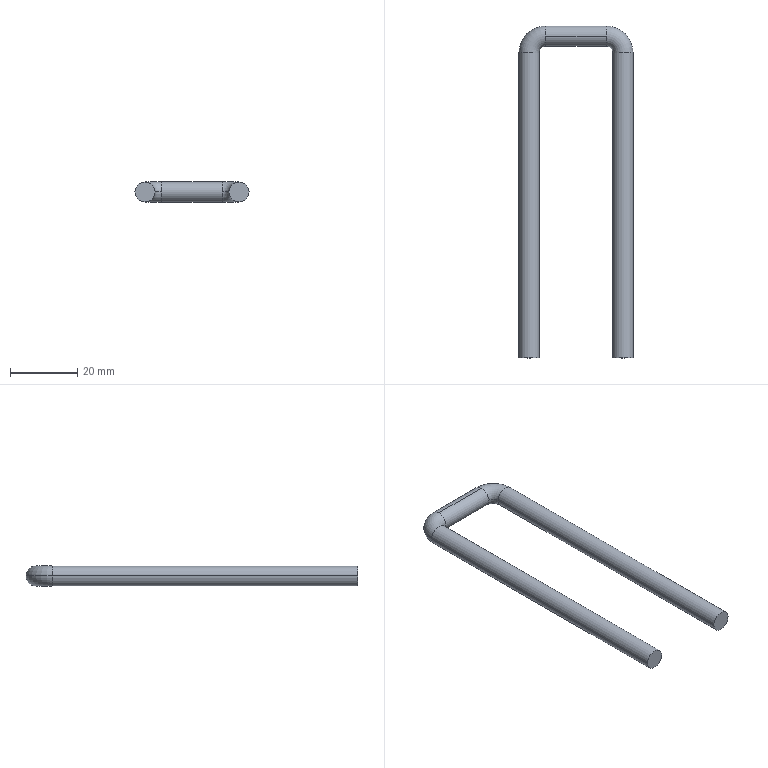Part | SolidWorks | features Sweep 1 | 1 solid | 12 faces | box 34 x 99 x 6 mm | volume 6099 mm3 | cylinder 6 | torus 4 | plane 2 | commonest cylinder face diameters 6 x6
STEP:
#1=CARTESIAN_POINT('',(-11.,91.,0.));
#2=VERTEX_POINT('',#1);
#3=CARTESIAN_POINT('',(-17.,91.,0.));
#4=VERTEX_POINT('',#3);
#5=CARTESIAN_POINT('',(-14.,91.,0.));
#6=DIRECTION('',(0.,1.,0.));
#7=DIRECTION('',(0.,0.,1.));
#8=AXIS2_PLACEMENT_3D('',#5,#6,#7);
#9=CIRCLE('',#8,3.);
#10=EDGE_CURVE('',#2,#4,#9,.T.);
#11=ORIENTED_EDGE('',*,*,#10,.T.);
#12=CARTESIAN_POINT('',(-9.,99.,0.));
#13=VERTEX_POINT('',#12);
#14=CARTESIAN_POINT('',(-9.,91.,0.));
#15=DIRECTION('',(0.,0.,-1.));
#16=DIRECTION('',(0.,1.,0.));
#17=AXIS2_PLACEMENT_3D('',#14,#15,#16);
#18=CIRCLE('',#17,8.);
#19=EDGE_CURVE('',#4,#13,#18,.T.);
#20=ORIENTED_EDGE('',*,*,#19,.T.);
#21=CARTESIAN_POINT('',(-9.,96.,-3.));
#22=VERTEX_POINT('',#21);
#23=CARTESIAN_POINT('',(-9.,96.,0.));
#24=DIRECTION('',(1.,0.,0.));
#25=DIRECTION('',(0.,0.,1.));
#26=AXIS2_PLACEMENT_3D('',#23,#24,#25);
#27=CIRCLE('',#26,3.);
#28=EDGE_CURVE('',#22,#13,#27,.T.);
#29=ORIENTED_EDGE('',*,*,#28,.F.);
#30=CARTESIAN_POINT('',(-9.,93.,0.));
#31=VERTEX_POINT('',#30);
#32=CARTESIAN_POINT('',(-9.,96.,0.));
#33=DIRECTION('',(1.,0.,0.));
#34=DIRECTION('',(0.,0.,1.));
#35=AXIS2_PLACEMENT_3D('',#32,#33,#34);
#36=CIRCLE('',#35,3.);
#37=EDGE_CURVE('',#31,#22,#36,.T.);
#38=ORIENTED_EDGE('',*,*,#37,.F.);
#39=CARTESIAN_POINT('',(-9.,91.,0.));
#40=DIRECTION('',(0.,0.,-1.));
#41=DIRECTION('',(0.,1.,0.));
#42=AXIS2_PLACEMENT_3D('',#39,#40,#41);
#43=CIRCLE('',#42,2.);
#44=EDGE_CURVE('',#2,#31,#43,.T.);
#45=ORIENTED_EDGE('',*,*,#44,.F.);
#46=EDGE_LOOP('',(#11,#20,#29,#38,#45));
#47=FACE_OUTER_BOUND('',#46,.T.);
#48=CARTESIAN_POINT('',(-9.,91.,0.));
#49=DIRECTION('',(0.,0.,-1.));
#50=DIRECTION('',(-1.,0.,0.));
#51=AXIS2_PLACEMENT_3D('',#48,#49,#50);
#52=TOROIDAL_SURFACE('',#51,5.,3.);
#53=ADVANCED_FACE('',(#47),#52,.T.);
#54=CARTESIAN_POINT('',(9.,96.,-3.));
#55=VERTEX_POINT('',#54);
#56=CARTESIAN_POINT('',(9.,99.,0.));
#57=VERTEX_POINT('',#56);
#58=CARTESIAN_POINT('',(9.,96.,0.));
#59=DIRECTION('',(1.,0.,0.));
#60=DIRECTION('',(0.,0.,1.));
#61=AXIS2_PLACEMENT_3D('',#58,#59,#60);
#62=CIRCLE('',#61,3.);
#63=EDGE_CURVE('',#55,#57,#62,.T.);
#64=ORIENTED_EDGE('',*,*,#63,.T.);
#65=CARTESIAN_POINT('',(17.,91.,0.));
#66=VERTEX_POINT('',#65);
#67=CARTESIAN_POINT('',(9.,91.,0.));
#68=DIRECTION('',(0.,0.,-1.));
#69=DIRECTION('',(0.,1.,0.));
#70=AXIS2_PLACEMENT_3D('',#67,#68,#69);
#71=CIRCLE('',#70,8.);
#72=EDGE_CURVE('',#57,#66,#71,.T.);
#73=ORIENTED_EDGE('',*,*,#72,.T.);
#74=CARTESIAN_POINT('',(11.,91.,0.));
#75=VERTEX_POINT('',#74);
#76=CARTESIAN_POINT('',(14.,91.,0.));
#77=DIRECTION('',(0.,-1.,0.));
#78=DIRECTION('',(0.,0.,1.));
#79=AXIS2_PLACEMENT_3D('',#76,#77,#78);
#80=CIRCLE('',#79,3.);
#81=EDGE_CURVE('',#75,#66,#80,.T.);
#82=ORIENTED_EDGE('',*,*,#81,.F.);
#83=CARTESIAN_POINT('',(9.,93.,0.));
#84=VERTEX_POINT('',#83);
#85=CARTESIAN_POINT('',(9.,91.,0.));
#86=DIRECTION('',(0.,0.,-1.));
#87=DIRECTION('',(0.,1.,0.));
#88=AXIS2_PLACEMENT_3D('',#85,#86,#87);
#89=CIRCLE('',#88,2.);
#90=EDGE_CURVE('',#84,#75,#89,.T.);
#91=ORIENTED_EDGE('',*,*,#90,.F.);
#92=CARTESIAN_POINT('',(9.,96.,0.));
#93=DIRECTION('',(1.,0.,0.));
#94=DIRECTION('',(0.,0.,1.));
#95=AXIS2_PLACEMENT_3D('',#92,#93,#94);
#96=CIRCLE('',#95,3.);
#97=EDGE_CURVE('',#84,#55,#96,.T.);
#98=ORIENTED_EDGE('',*,*,#97,.T.);
#99=EDGE_LOOP('',(#64,#73,#82,#91,#98));
#100=FACE_OUTER_BOUND('',#99,.T.);
#101=CARTESIAN_POINT('',(9.,91.,0.));
#102=DIRECTION('',(0.,0.,-1.));
#103=DIRECTION('',(-1.,0.,0.));
#104=AXIS2_PLACEMENT_3D('',#101,#102,#103);
#105=TOROIDAL_SURFACE('',#104,5.,3.);
#106=ADVANCED_FACE('',(#100),#105,.T.);
#107=CARTESIAN_POINT('',(-14.,91.,0.));
#108=DIRECTION('',(0.,1.,0.));
#109=DIRECTION('',(0.,0.,1.));
#110=AXIS2_PLACEMENT_3D('',#107,#108,#109);
#111=CIRCLE('',#110,3.);
#112=EDGE_CURVE('',#4,#2,#111,.T.);
#113=ORIENTED_EDGE('',*,*,#112,.F.);
#114=CARTESIAN_POINT('',(-17.,0.,0.));
#115=VERTEX_POINT('',#114);
#116=CARTESIAN_POINT('',(-17.,91.,0.));
#117=DIRECTION('',(0.,-1.,0.));
#118=VECTOR('',#117,1000.);
#119=LINE('',#116,#118);
#120=EDGE_CURVE('',#4,#115,#119,.T.);
#121=ORIENTED_EDGE('',*,*,#120,.T.);
#122=CARTESIAN_POINT('',(-11.,0.,0.));
#123=VERTEX_POINT('',#122);
#124=CARTESIAN_POINT('',(-14.,0.,0.));
#125=DIRECTION('',(0.,1.,0.));
#126=DIRECTION('',(0.,0.,1.));
#127=AXIS2_PLACEMENT_3D('',#124,#125,#126);
#128=CIRCLE('',#127,3.);
#129=EDGE_CURVE('',#115,#123,#128,.T.);
#130=ORIENTED_EDGE('',*,*,#129,.T.);
#131=CARTESIAN_POINT('',(-11.,91.,0.));
#132=DIRECTION('',(0.,-1.,0.));
#133=VECTOR('',#132,1000.);
#134=LINE('',#131,#133);
#135=EDGE_CURVE('',#2,#123,#134,.T.);
#136=ORIENTED_EDGE('',*,*,#135,.F.);
#137=EDGE_LOOP('',(#113,#121,#130,#136));
#138=FACE_OUTER_BOUND('',#137,.T.);
#139=CARTESIAN_POINT('',(-14.,91.,0.));
#140=DIRECTION('',(0.,-1.,0.));
#141=DIRECTION('',(1.,0.,0.));
#142=AXIS2_PLACEMENT_3D('',#139,#140,#141);
#143=CYLINDRICAL_SURFACE('',#142,3.);
#144=ADVANCED_FACE('',(#138),#143,.T.);
#145=ORIENTED_EDGE('',*,*,#28,.T.);
#146=CARTESIAN_POINT('',(-9.,96.,3.));
#147=VERTEX_POINT('',#146);
#148=CARTESIAN_POINT('',(-9.,96.,0.));
#149=DIRECTION('',(1.,0.,0.));
#150=DIRECTION('',(0.,0.,1.));
#151=AXIS2_PLACEMENT_3D('',#148,#149,#150);
#152=CIRCLE('',#151,3.);
#153=EDGE_CURVE('',#13,#147,#152,.T.);
#154=ORIENTED_EDGE('',*,*,#153,.T.);
#155=CARTESIAN_POINT('',(9.,96.,3.));
#156=VERTEX_POINT('',#155);
#157=CARTESIAN_POINT('',(-9.,96.,3.));
#158=DIRECTION('',(1.,0.,0.));
#159=VECTOR('',#158,1000.);
#160=LINE('',#157,#159);
#161=EDGE_CURVE('',#147,#156,#160,.T.);
#162=ORIENTED_EDGE('',*,*,#161,.T.);
#163=CARTESIAN_POINT('',(9.,96.,0.));
#164=DIRECTION('',(1.,0.,0.));
#165=DIRECTION('',(0.,0.,1.));
#166=AXIS2_PLACEMENT_3D('',#163,#164,#165);
#167=CIRCLE('',#166,3.);
#168=EDGE_CURVE('',#57,#156,#167,.T.);
#169=ORIENTED_EDGE('',*,*,#168,.F.);
#170=ORIENTED_EDGE('',*,*,#63,.F.);
#171=CARTESIAN_POINT('',(-9.,96.,-3.));
#172=DIRECTION('',(1.,0.,0.));
#173=VECTOR('',#172,1000.);
#174=LINE('',#171,#173);
#175=EDGE_CURVE('',#22,#55,#174,.T.);
#176=ORIENTED_EDGE('',*,*,#175,.F.);
#177=EDGE_LOOP('',(#145,#154,#162,#169,#170,#176));
#178=FACE_OUTER_BOUND('',#177,.T.);
#179=CARTESIAN_POINT('',(-9.,96.,0.));
#180=DIRECTION('',(1.,0.,0.));
#181=DIRECTION('',(0.,0.,-1.));
#182=AXIS2_PLACEMENT_3D('',#179,#180,#181);
#183=CYLINDRICAL_SURFACE('',#182,3.);
#184=ADVANCED_FACE('',(#178),#183,.T.);
#185=CARTESIAN_POINT('',(14.,91.,0.));
#186=DIRECTION('',(0.,-1.,0.));
#187=DIRECTION('',(0.,0.,1.));
#188=AXIS2_PLACEMENT_3D('',#185,#186,#187);
#189=CIRCLE('',#188,3.);
#190=EDGE_CURVE('',#66,#75,#189,.T.);
#191=ORIENTED_EDGE('',*,*,#190,.T.);
#192=CARTESIAN_POINT('',(11.,0.,0.));
#193=VERTEX_POINT('',#192);
#194=CARTESIAN_POINT('',(11.,91.,0.));
#195=DIRECTION('',(0.,-1.,0.));
#196=VECTOR('',#195,1000.);
#197=LINE('',#194,#196);
#198=EDGE_CURVE('',#75,#193,#197,.T.);
#199=ORIENTED_EDGE('',*,*,#198,.T.);
#200=CARTESIAN_POINT('',(17.,0.,0.));
#201=VERTEX_POINT('',#200);
#202=CARTESIAN_POINT('',(14.,0.,0.));
#203=DIRECTION('',(0.,-1.,0.));
#204=DIRECTION('',(0.,0.,1.));
#205=AXIS2_PLACEMENT_3D('',#202,#203,#204);
#206=CIRCLE('',#205,3.);
#207=EDGE_CURVE('',#201,#193,#206,.T.);
#208=ORIENTED_EDGE('',*,*,#207,.F.);
#209=CARTESIAN_POINT('',(17.,91.,0.));
#210=DIRECTION('',(0.,-1.,0.));
#211=VECTOR('',#210,1000.);
#212=LINE('',#209,#211);
#213=EDGE_CURVE('',#66,#201,#212,.T.);
#214=ORIENTED_EDGE('',*,*,#213,.F.);
#215=EDGE_LOOP('',(#191,#199,#208,#214));
#216=FACE_OUTER_BOUND('',#215,.T.);
#217=CARTESIAN_POINT('',(14.,91.,0.));
#218=DIRECTION('',(0.,-1.,0.));
#219=DIRECTION('',(1.,0.,0.));
#220=AXIS2_PLACEMENT_3D('',#217,#218,#219);
#221=CYLINDRICAL_SURFACE('',#220,3.);
#222=ADVANCED_FACE('',(#216),#221,.T.);
#223=ORIENTED_EDGE('',*,*,#198,.F.);
#224=ORIENTED_EDGE('',*,*,#81,.T.);
#225=ORIENTED_EDGE('',*,*,#213,.T.);
#226=CARTESIAN_POINT('',(14.,0.,0.));
#227=DIRECTION('',(0.,-1.,0.));
#228=DIRECTION('',(0.,0.,1.));
#229=AXIS2_PLACEMENT_3D('',#226,#227,#228);
#230=CIRCLE('',#229,3.);
#231=EDGE_CURVE('',#193,#201,#230,.T.);
#232=ORIENTED_EDGE('',*,*,#231,.F.);
#233=EDGE_LOOP('',(#223,#224,#225,#232));
#234=FACE_OUTER_BOUND('',#233,.T.);
#235=CARTESIAN_POINT('',(14.,91.,0.));
#236=DIRECTION('',(0.,-1.,0.));
#237=DIRECTION('',(1.,0.,0.));
#238=AXIS2_PLACEMENT_3D('',#235,#236,#237);
#239=CYLINDRICAL_SURFACE('',#238,3.);
#240=ADVANCED_FACE('',(#234),#239,.T.);
#241=ORIENTED_EDGE('',*,*,#72,.F.);
#242=ORIENTED_EDGE('',*,*,#168,.T.);
#243=CARTESIAN_POINT('',(9.,96.,0.));
#244=DIRECTION('',(1.,0.,0.));
#245=DIRECTION('',(0.,0.,1.));
#246=AXIS2_PLACEMENT_3D('',#243,#244,#245);
#247=CIRCLE('',#246,3.);
#248=EDGE_CURVE('',#156,#84,#247,.T.);
#249=ORIENTED_EDGE('',*,*,#248,.T.);
#250=ORIENTED_EDGE('',*,*,#90,.T.);
#251=ORIENTED_EDGE('',*,*,#190,.F.);
#252=EDGE_LOOP('',(#241,#242,#249,#250,#251));
#253=FACE_OUTER_BOUND('',#252,.T.);
#254=CARTESIAN_POINT('',(9.,91.,0.));
#255=DIRECTION('',(0.,0.,-1.));
#256=DIRECTION('',(-1.,0.,0.));
#257=AXIS2_PLACEMENT_3D('',#254,#255,#256);
#258=TOROIDAL_SURFACE('',#257,5.,3.);
#259=ADVANCED_FACE('',(#253),#258,.T.);
#260=ORIENTED_EDGE('',*,*,#161,.F.);
#261=CARTESIAN_POINT('',(-9.,96.,0.));
#262=DIRECTION('',(1.,0.,0.));
#263=DIRECTION('',(0.,0.,1.));
#264=AXIS2_PLACEMENT_3D('',#261,#262,#263);
#265=CIRCLE('',#264,3.);
#266=EDGE_CURVE('',#147,#31,#265,.T.);
#267=ORIENTED_EDGE('',*,*,#266,.T.);
#268=ORIENTED_EDGE('',*,*,#37,.T.);
#269=ORIENTED_EDGE('',*,*,#175,.T.);
#270=ORIENTED_EDGE('',*,*,#97,.F.);
#271=ORIENTED_EDGE('',*,*,#248,.F.);
#272=EDGE_LOOP('',(#260,#267,#268,#269,#270,#271));
#273=FACE_OUTER_BOUND('',#272,.T.);
#274=CARTESIAN_POINT('',(-9.,96.,0.));
#275=DIRECTION('',(1.,0.,0.));
#276=DIRECTION('',(0.,0.,-1.));
#277=AXIS2_PLACEMENT_3D('',#274,#275,#276);
#278=CYLINDRICAL_SURFACE('',#277,3.);
#279=ADVANCED_FACE('',(#273),#278,.T.);
#280=ORIENTED_EDGE('',*,*,#19,.F.);
#281=ORIENTED_EDGE('',*,*,#112,.T.);
#282=ORIENTED_EDGE('',*,*,#44,.T.);
#283=ORIENTED_EDGE('',*,*,#266,.F.);
#284=ORIENTED_EDGE('',*,*,#153,.F.);
#285=EDGE_LOOP('',(#280,#281,#282,#283,#284));
#286=FACE_OUTER_BOUND('',#285,.T.);
#287=CARTESIAN_POINT('',(-9.,91.,0.));
#288=DIRECTION('',(0.,0.,-1.));
#289=DIRECTION('',(-1.,0.,0.));
#290=AXIS2_PLACEMENT_3D('',#287,#288,#289);
#291=TOROIDAL_SURFACE('',#290,5.,3.);
#292=ADVANCED_FACE('',(#286),#291,.T.);
#293=ORIENTED_EDGE('',*,*,#120,.F.);
#294=ORIENTED_EDGE('',*,*,#10,.F.);
#295=ORIENTED_EDGE('',*,*,#135,.T.);
#296=CARTESIAN_POINT('',(-14.,0.,0.));
#297=DIRECTION('',(0.,1.,0.));
#298=DIRECTION('',(0.,0.,1.));
#299=AXIS2_PLACEMENT_3D('',#296,#297,#298);
#300=CIRCLE('',#299,3.);
#301=EDGE_CURVE('',#123,#115,#300,.T.);
#302=ORIENTED_EDGE('',*,*,#301,.T.);
#303=EDGE_LOOP('',(#293,#294,#295,#302));
#304=FACE_OUTER_BOUND('',#303,.T.);
#305=CARTESIAN_POINT('',(-14.,91.,0.));
#306=DIRECTION('',(0.,-1.,0.));
#307=DIRECTION('',(1.,0.,0.));
#308=AXIS2_PLACEMENT_3D('',#305,#306,#307);
#309=CYLINDRICAL_SURFACE('',#308,3.);
#310=ADVANCED_FACE('',(#304),#309,.T.);
#311=ORIENTED_EDGE('',*,*,#207,.T.);
#312=ORIENTED_EDGE('',*,*,#231,.T.);
#313=EDGE_LOOP('',(#311,#312));
#314=FACE_OUTER_BOUND('',#313,.T.);
#315=CARTESIAN_POINT('',(14.,0.,0.));
#316=DIRECTION('',(0.,-1.,0.));
#317=DIRECTION('',(0.,0.,1.));
#318=AXIS2_PLACEMENT_3D('',#315,#316,#317);
#319=PLANE('',#318);
#320=ADVANCED_FACE('',(#314),#319,.T.);
#321=ORIENTED_EDGE('',*,*,#301,.F.);
#322=ORIENTED_EDGE('',*,*,#129,.F.);
#323=EDGE_LOOP('',(#321,#322));
#324=FACE_OUTER_BOUND('',#323,.T.);
#325=CARTESIAN_POINT('',(-14.,0.,0.));
#326=DIRECTION('',(0.,1.,0.));
#327=DIRECTION('',(0.,0.,1.));
#328=AXIS2_PLACEMENT_3D('',#325,#326,#327);
#329=PLANE('',#328);
#330=ADVANCED_FACE('',(#324),#329,.F.);
#331=CLOSED_SHELL('',(#53,#106,#144,#184,#222,#240,#259,#279,#292,#310,#320,#330));
#332=MANIFOLD_SOLID_BREP('',#331);
#333=CARTESIAN_POINT('',(0.,0.,0.));
#334=DIRECTION('',(0.,0.,1.));
#335=DIRECTION('',(1.,0.,0.));
#336=AXIS2_PLACEMENT_3D('',#333,#334,#335);
#337=(LENGTH_UNIT()NAMED_UNIT(*)SI_UNIT(.MILLI.,.METRE.));
#338=UNCERTAINTY_MEASURE_WITH_UNIT(LENGTH_MEASURE(0.00001),#337,'','');
#339=(NAMED_UNIT(*)PLANE_ANGLE_UNIT()SI_UNIT($,.RADIAN.));
#340=(NAMED_UNIT(*)SI_UNIT($,.STERADIAN.)SOLID_ANGLE_UNIT());
#341=(GEOMETRIC_REPRESENTATION_CONTEXT(3)GLOBAL_UNCERTAINTY_ASSIGNED_CONTEXT((#338))GLOBAL_UNIT_ASSIGNED_CONTEXT((#337,#339,#340))REPRESENTATION_CONTEXT('',''));
#342=ADVANCED_BREP_SHAPE_REPRESENTATION('',(#332,#336),#341);